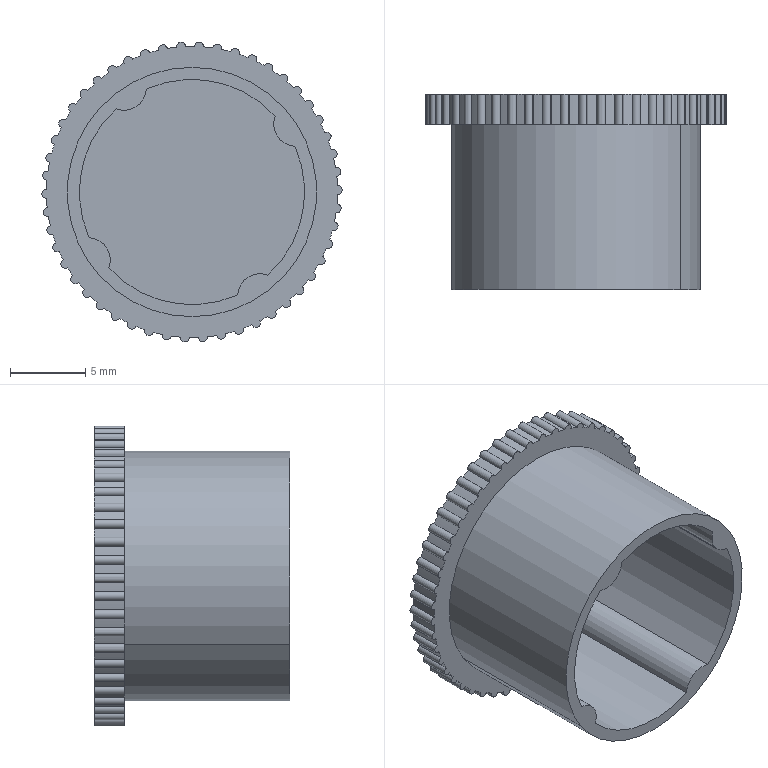Part | SolidWorks | features BaseBody 1 | 1 solid | 144 faces | box 19.998 x 13 x 19.976 mm | volume 921.635 mm3 | cylinder 140 | plane 4 | commonest cylinder face diameters 0.6 x78 19.4 x51 3 x5 15 x4 16.6 x2